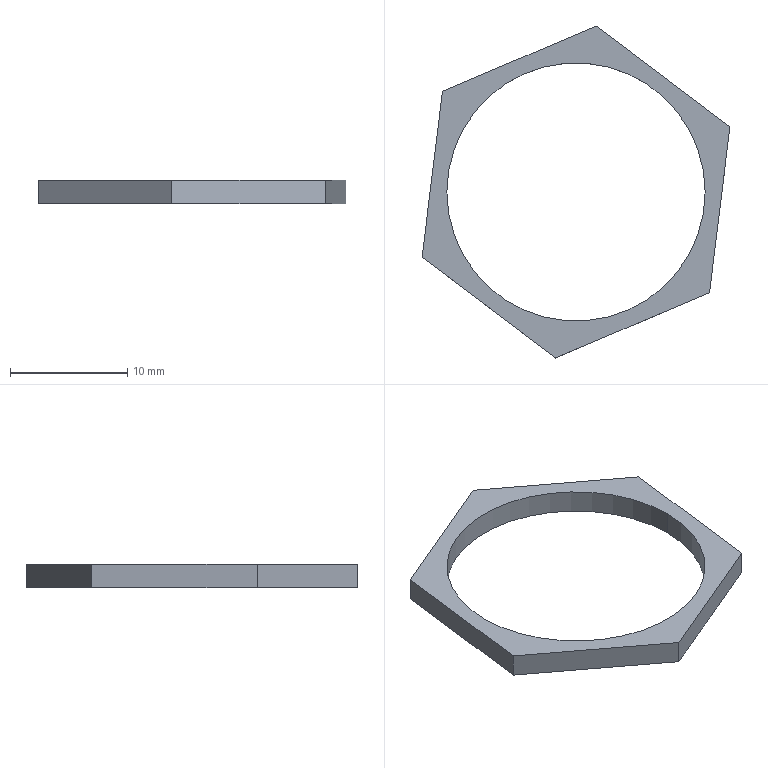Part | SolidWorks | features Extrusion 1 | 1 solid | 10 faces | box 26.237 x 28.287 x 2 mm | volume 294.878 mm3 | plane 8 | cylinder 2 | commonest cylinder face diameters 22 x2
STEP:
#1=CARTESIAN_POINT('',(-12.485,26.053,2.));
#2=VERTEX_POINT('',#1);
#3=CARTESIAN_POINT('',(9.515,26.053,2.));
#4=VERTEX_POINT('',#3);
#5=CARTESIAN_POINT('',(-1.485,26.053,2.));
#6=DIRECTION('',(0.,0.,1.));
#7=DIRECTION('',(1.,0.,0.));
#8=AXIS2_PLACEMENT_3D('',#5,#6,#7);
#9=CIRCLE('',#8,11.);
#10=EDGE_CURVE('',#2,#4,#9,.T.);
#11=ORIENTED_EDGE('',*,*,#10,.T.);
#12=CARTESIAN_POINT('',(9.515,26.053,0.));
#13=VERTEX_POINT('',#12);
#14=CARTESIAN_POINT('',(9.515,26.053,2.));
#15=DIRECTION('',(0.,0.,-1.));
#16=VECTOR('',#15,1000.);
#17=LINE('',#14,#16);
#18=EDGE_CURVE('',#4,#13,#17,.T.);
#19=ORIENTED_EDGE('',*,*,#18,.T.);
#20=CARTESIAN_POINT('',(-12.485,26.053,0.));
#21=VERTEX_POINT('',#20);
#22=CARTESIAN_POINT('',(-1.485,26.053,0.));
#23=DIRECTION('',(0.,0.,1.));
#24=DIRECTION('',(1.,0.,0.));
#25=AXIS2_PLACEMENT_3D('',#22,#23,#24);
#26=CIRCLE('',#25,11.);
#27=EDGE_CURVE('',#21,#13,#26,.T.);
#28=ORIENTED_EDGE('',*,*,#27,.F.);
#29=CARTESIAN_POINT('',(-12.485,26.053,2.));
#30=DIRECTION('',(0.,0.,-1.));
#31=VECTOR('',#30,1000.);
#32=LINE('',#29,#31);
#33=EDGE_CURVE('',#2,#21,#32,.T.);
#34=ORIENTED_EDGE('',*,*,#33,.F.);
#35=EDGE_LOOP('',(#11,#19,#28,#34));
#36=FACE_OUTER_BOUND('',#35,.T.);
#37=CARTESIAN_POINT('',(-1.485,26.053,2.));
#38=DIRECTION('',(0.,0.,-1.));
#39=DIRECTION('',(-1.,0.,0.));
#40=AXIS2_PLACEMENT_3D('',#37,#38,#39);
#41=CYLINDRICAL_SURFACE('',#40,11.);
#42=ADVANCED_FACE('',(#36),#41,.F.);
#43=CARTESIAN_POINT('',(-3.225,11.91,2.));
#44=VERTEX_POINT('',#43);
#45=CARTESIAN_POINT('',(9.893,17.474,2.));
#46=VERTEX_POINT('',#45);
#47=CARTESIAN_POINT('',(-3.225,11.91,2.));
#48=DIRECTION('',(0.9206,0.3905,0.));
#49=VECTOR('',#48,1000.);
#50=LINE('',#47,#49);
#51=EDGE_CURVE('',#44,#46,#50,.T.);
#52=ORIENTED_EDGE('',*,*,#51,.T.);
#53=CARTESIAN_POINT('',(11.634,31.617,2.));
#54=VERTEX_POINT('',#53);
#55=CARTESIAN_POINT('',(9.893,17.474,2.));
#56=DIRECTION('',(0.1221,0.9925,0.));
#57=VECTOR('',#56,1000.);
#58=LINE('',#55,#57);
#59=EDGE_CURVE('',#46,#54,#58,.T.);
#60=ORIENTED_EDGE('',*,*,#59,.T.);
#61=CARTESIAN_POINT('',(0.2553,40.196,2.));
#62=VERTEX_POINT('',#61);
#63=CARTESIAN_POINT('',(11.634,31.617,2.));
#64=DIRECTION('',(-0.7985,0.602,0.));
#65=VECTOR('',#64,1000.);
#66=LINE('',#63,#65);
#67=EDGE_CURVE('',#54,#62,#66,.T.);
#68=ORIENTED_EDGE('',*,*,#67,.T.);
#69=CARTESIAN_POINT('',(-12.863,34.632,2.));
#70=VERTEX_POINT('',#69);
#71=CARTESIAN_POINT('',(0.2553,40.196,2.));
#72=DIRECTION('',(-0.9206,-0.3905,0.));
#73=VECTOR('',#72,1000.);
#74=LINE('',#71,#73);
#75=EDGE_CURVE('',#62,#70,#74,.T.);
#76=ORIENTED_EDGE('',*,*,#75,.T.);
#77=CARTESIAN_POINT('',(-14.604,20.489,2.));
#78=VERTEX_POINT('',#77);
#79=CARTESIAN_POINT('',(-12.863,34.632,2.));
#80=DIRECTION('',(-0.1221,-0.9925,0.));
#81=VECTOR('',#80,1000.);
#82=LINE('',#79,#81);
#83=EDGE_CURVE('',#70,#78,#82,.T.);
#84=ORIENTED_EDGE('',*,*,#83,.T.);
#85=CARTESIAN_POINT('',(-14.604,20.489,2.));
#86=DIRECTION('',(0.7985,-0.602,0.));
#87=VECTOR('',#86,1000.);
#88=LINE('',#85,#87);
#89=EDGE_CURVE('',#78,#44,#88,.T.);
#90=ORIENTED_EDGE('',*,*,#89,.T.);
#91=EDGE_LOOP('',(#52,#60,#68,#76,#84,#90));
#92=FACE_OUTER_BOUND('',#91,.T.);
#93=ORIENTED_EDGE('',*,*,#10,.F.);
#94=CARTESIAN_POINT('',(-1.485,26.053,2.));
#95=DIRECTION('',(0.,0.,1.));
#96=DIRECTION('',(1.,0.,0.));
#97=AXIS2_PLACEMENT_3D('',#94,#95,#96);
#98=CIRCLE('',#97,11.);
#99=EDGE_CURVE('',#4,#2,#98,.T.);
#100=ORIENTED_EDGE('',*,*,#99,.F.);
#101=EDGE_LOOP('',(#93,#100));
#102=FACE_BOUND('',#101,.T.);
#103=CARTESIAN_POINT('',(0.,0.,2.));
#104=DIRECTION('',(0.,0.,1.));
#105=DIRECTION('',(1.,0.,0.));
#106=AXIS2_PLACEMENT_3D('',#103,#104,#105);
#107=PLANE('',#106);
#108=ADVANCED_FACE('',(#92,#102),#107,.T.);
#109=CARTESIAN_POINT('',(-3.225,11.91,0.));
#110=VERTEX_POINT('',#109);
#111=CARTESIAN_POINT('',(9.893,17.474,0.));
#112=VERTEX_POINT('',#111);
#113=CARTESIAN_POINT('',(-3.225,11.91,0.));
#114=DIRECTION('',(0.9206,0.3905,0.));
#115=VECTOR('',#114,1000.);
#116=LINE('',#113,#115);
#117=EDGE_CURVE('',#110,#112,#116,.T.);
#118=ORIENTED_EDGE('',*,*,#117,.F.);
#119=CARTESIAN_POINT('',(-14.604,20.489,0.));
#120=VERTEX_POINT('',#119);
#121=CARTESIAN_POINT('',(-14.604,20.489,0.));
#122=DIRECTION('',(0.7985,-0.602,0.));
#123=VECTOR('',#122,1000.);
#124=LINE('',#121,#123);
#125=EDGE_CURVE('',#120,#110,#124,.T.);
#126=ORIENTED_EDGE('',*,*,#125,.F.);
#127=CARTESIAN_POINT('',(-12.863,34.632,0.));
#128=VERTEX_POINT('',#127);
#129=CARTESIAN_POINT('',(-12.863,34.632,0.));
#130=DIRECTION('',(-0.1221,-0.9925,0.));
#131=VECTOR('',#130,1000.);
#132=LINE('',#129,#131);
#133=EDGE_CURVE('',#128,#120,#132,.T.);
#134=ORIENTED_EDGE('',*,*,#133,.F.);
#135=CARTESIAN_POINT('',(0.2553,40.196,0.));
#136=VERTEX_POINT('',#135);
#137=CARTESIAN_POINT('',(0.2553,40.196,0.));
#138=DIRECTION('',(-0.9206,-0.3905,0.));
#139=VECTOR('',#138,1000.);
#140=LINE('',#137,#139);
#141=EDGE_CURVE('',#136,#128,#140,.T.);
#142=ORIENTED_EDGE('',*,*,#141,.F.);
#143=CARTESIAN_POINT('',(11.634,31.617,0.));
#144=VERTEX_POINT('',#143);
#145=CARTESIAN_POINT('',(11.634,31.617,0.));
#146=DIRECTION('',(-0.7985,0.602,0.));
#147=VECTOR('',#146,1000.);
#148=LINE('',#145,#147);
#149=EDGE_CURVE('',#144,#136,#148,.T.);
#150=ORIENTED_EDGE('',*,*,#149,.F.);
#151=CARTESIAN_POINT('',(9.893,17.474,0.));
#152=DIRECTION('',(0.1221,0.9925,0.));
#153=VECTOR('',#152,1000.);
#154=LINE('',#151,#153);
#155=EDGE_CURVE('',#112,#144,#154,.T.);
#156=ORIENTED_EDGE('',*,*,#155,.F.);
#157=EDGE_LOOP('',(#118,#126,#134,#142,#150,#156));
#158=FACE_OUTER_BOUND('',#157,.T.);
#159=ORIENTED_EDGE('',*,*,#27,.T.);
#160=CARTESIAN_POINT('',(-1.485,26.053,0.));
#161=DIRECTION('',(0.,0.,1.));
#162=DIRECTION('',(1.,0.,0.));
#163=AXIS2_PLACEMENT_3D('',#160,#161,#162);
#164=CIRCLE('',#163,11.);
#165=EDGE_CURVE('',#13,#21,#164,.T.);
#166=ORIENTED_EDGE('',*,*,#165,.T.);
#167=EDGE_LOOP('',(#159,#166));
#168=FACE_BOUND('',#167,.T.);
#169=CARTESIAN_POINT('',(0.,0.,0.));
#170=DIRECTION('',(0.,0.,1.));
#171=DIRECTION('',(1.,0.,0.));
#172=AXIS2_PLACEMENT_3D('',#169,#170,#171);
#173=PLANE('',#172);
#174=ADVANCED_FACE('',(#158,#168),#173,.F.);
#175=ORIENTED_EDGE('',*,*,#117,.T.);
#176=CARTESIAN_POINT('',(9.893,17.474,2.));
#177=DIRECTION('',(0.,0.,-1.));
#178=VECTOR('',#177,1000.);
#179=LINE('',#176,#178);
#180=EDGE_CURVE('',#46,#112,#179,.T.);
#181=ORIENTED_EDGE('',*,*,#180,.F.);
#182=ORIENTED_EDGE('',*,*,#51,.F.);
#183=CARTESIAN_POINT('',(-3.225,11.91,2.));
#184=DIRECTION('',(0.,0.,-1.));
#185=VECTOR('',#184,1000.);
#186=LINE('',#183,#185);
#187=EDGE_CURVE('',#44,#110,#186,.T.);
#188=ORIENTED_EDGE('',*,*,#187,.T.);
#189=EDGE_LOOP('',(#175,#181,#182,#188));
#190=FACE_OUTER_BOUND('',#189,.T.);
#191=CARTESIAN_POINT('',(-3.225,11.91,2.));
#192=DIRECTION('',(-0.3905,0.9206,0.));
#193=DIRECTION('',(-0.9206,-0.3905,0.));
#194=AXIS2_PLACEMENT_3D('',#191,#192,#193);
#195=PLANE('',#194);
#196=ADVANCED_FACE('',(#190),#195,.F.);
#197=ORIENTED_EDGE('',*,*,#155,.T.);
#198=CARTESIAN_POINT('',(11.634,31.617,2.));
#199=DIRECTION('',(0.,0.,-1.));
#200=VECTOR('',#199,1000.);
#201=LINE('',#198,#200);
#202=EDGE_CURVE('',#54,#144,#201,.T.);
#203=ORIENTED_EDGE('',*,*,#202,.F.);
#204=ORIENTED_EDGE('',*,*,#59,.F.);
#205=ORIENTED_EDGE('',*,*,#180,.T.);
#206=EDGE_LOOP('',(#197,#203,#204,#205));
#207=FACE_OUTER_BOUND('',#206,.T.);
#208=CARTESIAN_POINT('',(9.893,17.474,2.));
#209=DIRECTION('',(-0.9925,0.1221,0.));
#210=DIRECTION('',(-0.1221,-0.9925,0.));
#211=AXIS2_PLACEMENT_3D('',#208,#209,#210);
#212=PLANE('',#211);
#213=ADVANCED_FACE('',(#207),#212,.F.);
#214=ORIENTED_EDGE('',*,*,#149,.T.);
#215=CARTESIAN_POINT('',(0.2553,40.196,2.));
#216=DIRECTION('',(0.,0.,-1.));
#217=VECTOR('',#216,1000.);
#218=LINE('',#215,#217);
#219=EDGE_CURVE('',#62,#136,#218,.T.);
#220=ORIENTED_EDGE('',*,*,#219,.F.);
#221=ORIENTED_EDGE('',*,*,#67,.F.);
#222=ORIENTED_EDGE('',*,*,#202,.T.);
#223=EDGE_LOOP('',(#214,#220,#221,#222));
#224=FACE_OUTER_BOUND('',#223,.T.);
#225=CARTESIAN_POINT('',(11.634,31.617,2.));
#226=DIRECTION('',(-0.602,-0.7985,0.));
#227=DIRECTION('',(0.7985,-0.602,0.));
#228=AXIS2_PLACEMENT_3D('',#225,#226,#227);
#229=PLANE('',#228);
#230=ADVANCED_FACE('',(#224),#229,.F.);
#231=ORIENTED_EDGE('',*,*,#141,.T.);
#232=CARTESIAN_POINT('',(-12.863,34.632,2.));
#233=DIRECTION('',(0.,0.,-1.));
#234=VECTOR('',#233,1000.);
#235=LINE('',#232,#234);
#236=EDGE_CURVE('',#70,#128,#235,.T.);
#237=ORIENTED_EDGE('',*,*,#236,.F.);
#238=ORIENTED_EDGE('',*,*,#75,.F.);
#239=ORIENTED_EDGE('',*,*,#219,.T.);
#240=EDGE_LOOP('',(#231,#237,#238,#239));
#241=FACE_OUTER_BOUND('',#240,.T.);
#242=CARTESIAN_POINT('',(0.2553,40.196,2.));
#243=DIRECTION('',(0.3905,-0.9206,0.));
#244=DIRECTION('',(0.9206,0.3905,0.));
#245=AXIS2_PLACEMENT_3D('',#242,#243,#244);
#246=PLANE('',#245);
#247=ADVANCED_FACE('',(#241),#246,.F.);
#248=ORIENTED_EDGE('',*,*,#133,.T.);
#249=CARTESIAN_POINT('',(-14.604,20.489,2.));
#250=DIRECTION('',(0.,0.,-1.));
#251=VECTOR('',#250,1000.);
#252=LINE('',#249,#251);
#253=EDGE_CURVE('',#78,#120,#252,.T.);
#254=ORIENTED_EDGE('',*,*,#253,.F.);
#255=ORIENTED_EDGE('',*,*,#83,.F.);
#256=ORIENTED_EDGE('',*,*,#236,.T.);
#257=EDGE_LOOP('',(#248,#254,#255,#256));
#258=FACE_OUTER_BOUND('',#257,.T.);
#259=CARTESIAN_POINT('',(-12.863,34.632,2.));
#260=DIRECTION('',(0.9925,-0.1221,0.));
#261=DIRECTION('',(0.1221,0.9925,0.));
#262=AXIS2_PLACEMENT_3D('',#259,#260,#261);
#263=PLANE('',#262);
#264=ADVANCED_FACE('',(#258),#263,.F.);
#265=ORIENTED_EDGE('',*,*,#125,.T.);
#266=ORIENTED_EDGE('',*,*,#187,.F.);
#267=ORIENTED_EDGE('',*,*,#89,.F.);
#268=ORIENTED_EDGE('',*,*,#253,.T.);
#269=EDGE_LOOP('',(#265,#266,#267,#268));
#270=FACE_OUTER_BOUND('',#269,.T.);
#271=CARTESIAN_POINT('',(-14.604,20.489,2.));
#272=DIRECTION('',(0.602,0.7985,0.));
#273=DIRECTION('',(-0.7985,0.602,0.));
#274=AXIS2_PLACEMENT_3D('',#271,#272,#273);
#275=PLANE('',#274);
#276=ADVANCED_FACE('',(#270),#275,.F.);
#277=ORIENTED_EDGE('',*,*,#18,.F.);
#278=ORIENTED_EDGE('',*,*,#99,.T.);
#279=ORIENTED_EDGE('',*,*,#33,.T.);
#280=ORIENTED_EDGE('',*,*,#165,.F.);
#281=EDGE_LOOP('',(#277,#278,#279,#280));
#282=FACE_OUTER_BOUND('',#281,.T.);
#283=CARTESIAN_POINT('',(-1.485,26.053,2.));
#284=DIRECTION('',(0.,0.,-1.));
#285=DIRECTION('',(-1.,0.,0.));
#286=AXIS2_PLACEMENT_3D('',#283,#284,#285);
#287=CYLINDRICAL_SURFACE('',#286,11.);
#288=ADVANCED_FACE('',(#282),#287,.F.);
#289=CLOSED_SHELL('',(#42,#108,#174,#196,#213,#230,#247,#264,#276,#288));
#290=MANIFOLD_SOLID_BREP('',#289);
#291=CARTESIAN_POINT('',(0.,0.,0.));
#292=DIRECTION('',(0.,0.,1.));
#293=DIRECTION('',(1.,0.,0.));
#294=AXIS2_PLACEMENT_3D('',#291,#292,#293);
#295=(LENGTH_UNIT()NAMED_UNIT(*)SI_UNIT(.MILLI.,.METRE.));
#296=UNCERTAINTY_MEASURE_WITH_UNIT(LENGTH_MEASURE(0.00001),#295,'','');
#297=(NAMED_UNIT(*)PLANE_ANGLE_UNIT()SI_UNIT($,.RADIAN.));
#298=(NAMED_UNIT(*)SI_UNIT($,.STERADIAN.)SOLID_ANGLE_UNIT());
#299=(GEOMETRIC_REPRESENTATION_CONTEXT(3)GLOBAL_UNCERTAINTY_ASSIGNED_CONTEXT((#296))GLOBAL_UNIT_ASSIGNED_CONTEXT((#295,#297,#298))REPRESENTATION_CONTEXT('',''));
#300=ADVANCED_BREP_SHAPE_REPRESENTATION('',(#290,#294),#299);